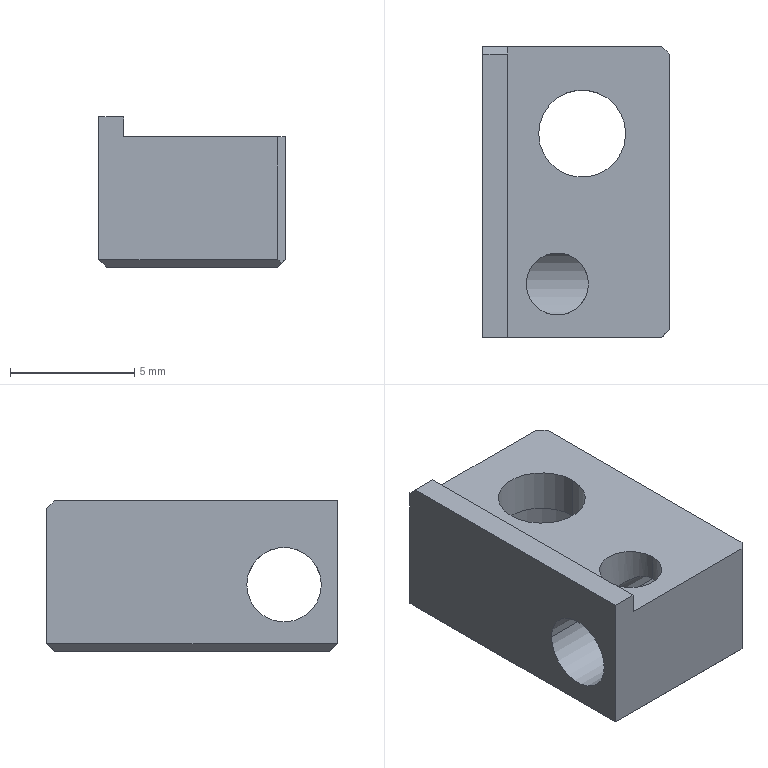Part | NX | 1 solid | 24 faces | box 7.5 x 11.687 x 6.04 mm | volume 291.783 mm3 | plane 16 | cylinder 8 | commonest cylinder face diameters 2.5 x2 3 x2 3.5 x2 6 x2
STEP:
#1=CARTESIAN_POINT('',(-53.86,-43.177,4.443));
#2=VERTEX_POINT('',#1);
#3=CARTESIAN_POINT('',(-51.36,-43.177,4.443));
#4=VERTEX_POINT('',#3);
#5=CARTESIAN_POINT('',(-52.61,-43.177,4.443));
#6=DIRECTION('',(0.,0.,1.));
#7=DIRECTION('',(1.,0.,0.));
#8=AXIS2_PLACEMENT_3D('',#5,#6,#7);
#9=CIRCLE('',#8,1.25);
#10=EDGE_CURVE('',#2,#4,#9,.T.);
#11=ORIENTED_EDGE('',*,*,#10,.T.);
#12=CARTESIAN_POINT('',(-51.36,-43.177,3.373));
#13=VERTEX_POINT('',#12);
#14=CARTESIAN_POINT('',(-51.36,-43.177,5.403));
#15=DIRECTION('',(0.,0.,1.));
#16=VECTOR('',#15,1000.);
#17=LINE('',#14,#16);
#18=EDGE_CURVE('',#13,#4,#17,.T.);
#19=ORIENTED_EDGE('',*,*,#18,.F.);
#20=CARTESIAN_POINT('',(-52.61,-44.427,2.702));
#21=VERTEX_POINT('',#20);
#22=CARTESIAN_POINT('',(-52.61,-44.427,2.702));
#23=CARTESIAN_POINT('',(-52.599,-44.427,2.702));
#24=CARTESIAN_POINT('',(-52.588,-44.426,2.702));
#25=CARTESIAN_POINT('',(-52.578,-44.426,2.703));
#26=CARTESIAN_POINT('',(-52.567,-44.426,2.703));
#27=CARTESIAN_POINT('',(-52.556,-44.425,2.704));
#28=CARTESIAN_POINT('',(-52.545,-44.425,2.705));
#29=CARTESIAN_POINT('',(-52.534,-44.424,2.706));
#30=CARTESIAN_POINT('',(-52.523,-44.424,2.707));
#31=CARTESIAN_POINT('',(-52.512,-44.423,2.708));
#32=CARTESIAN_POINT('',(-52.501,-44.422,2.709));
#33=CARTESIAN_POINT('',(-52.491,-44.421,2.711));
#34=CARTESIAN_POINT('',(-52.48,-44.42,2.712));
#35=CARTESIAN_POINT('',(-52.458,-44.418,2.716));
#36=CARTESIAN_POINT('',(-52.437,-44.415,2.72));
#37=CARTESIAN_POINT('',(-52.416,-44.411,2.725));
#38=CARTESIAN_POINT('',(-52.395,-44.408,2.73));
#39=CARTESIAN_POINT('',(-52.374,-44.404,2.735));
#40=CARTESIAN_POINT('',(-52.354,-44.4,2.741));
#41=CARTESIAN_POINT('',(-52.313,-44.391,2.753));
#42=CARTESIAN_POINT('',(-52.273,-44.381,2.768));
#43=CARTESIAN_POINT('',(-52.234,-44.369,2.784));
#44=CARTESIAN_POINT('',(-52.215,-44.363,2.792));
#45=CARTESIAN_POINT('',(-52.196,-44.356,2.8));
#46=CARTESIAN_POINT('',(-52.177,-44.349,2.809));
#47=CARTESIAN_POINT('',(-52.158,-44.342,2.817));
#48=CARTESIAN_POINT('',(-52.139,-44.335,2.826));
#49=CARTESIAN_POINT('',(-52.121,-44.327,2.836));
#50=CARTESIAN_POINT('',(-52.103,-44.319,2.845));
#51=CARTESIAN_POINT('',(-52.085,-44.311,2.854));
#52=CARTESIAN_POINT('',(-52.067,-44.303,2.864));
#53=CARTESIAN_POINT('',(-52.05,-44.294,2.874));
#54=CARTESIAN_POINT('',(-52.033,-44.285,2.884));
#55=CARTESIAN_POINT('',(-52.016,-44.276,2.893));
#56=CARTESIAN_POINT('',(-51.998,-44.267,2.903));
#57=CARTESIAN_POINT('',(-51.982,-44.257,2.913));
#58=CARTESIAN_POINT('',(-51.965,-44.247,2.924));
#59=CARTESIAN_POINT('',(-51.949,-44.237,2.934));
#60=CARTESIAN_POINT('',(-51.932,-44.227,2.944));
#61=CARTESIAN_POINT('',(-51.916,-44.216,2.954));
#62=CARTESIAN_POINT('',(-51.9,-44.205,2.965));
#63=CARTESIAN_POINT('',(-51.884,-44.194,2.975));
#64=CARTESIAN_POINT('',(-51.869,-44.183,2.985));
#65=CARTESIAN_POINT('',(-51.853,-44.171,2.996));
#66=CARTESIAN_POINT('',(-51.838,-44.16,3.006));
#67=CARTESIAN_POINT('',(-51.823,-44.147,3.017));
#68=CARTESIAN_POINT('',(-51.793,-44.123,3.037));
#69=CARTESIAN_POINT('',(-51.764,-44.097,3.058));
#70=CARTESIAN_POINT('',(-51.736,-44.07,3.078));
#71=CARTESIAN_POINT('',(-51.708,-44.043,3.098));
#72=CARTESIAN_POINT('',(-51.682,-44.014,3.118));
#73=CARTESIAN_POINT('',(-51.656,-43.985,3.137));
#74=CARTESIAN_POINT('',(-51.644,-43.97,3.146));
#75=CARTESIAN_POINT('',(-51.631,-43.954,3.156));
#76=CARTESIAN_POINT('',(-51.619,-43.939,3.165));
#77=CARTESIAN_POINT('',(-51.607,-43.923,3.174));
#78=CARTESIAN_POINT('',(-51.596,-43.907,3.183));
#79=CARTESIAN_POINT('',(-51.584,-43.891,3.192));
#80=CARTESIAN_POINT('',(-51.573,-43.874,3.201));
#81=CARTESIAN_POINT('',(-51.562,-43.857,3.21));
#82=CARTESIAN_POINT('',(-51.551,-43.84,3.218));
#83=CARTESIAN_POINT('',(-51.54,-43.823,3.227));
#84=CARTESIAN_POINT('',(-51.53,-43.806,3.235));
#85=CARTESIAN_POINT('',(-51.52,-43.788,3.243));
#86=CARTESIAN_POINT('',(-51.51,-43.77,3.251));
#87=CARTESIAN_POINT('',(-51.5,-43.752,3.259));
#88=CARTESIAN_POINT('',(-51.491,-43.733,3.266));
#89=CARTESIAN_POINT('',(-51.482,-43.715,3.273));
#90=CARTESIAN_POINT('',(-51.473,-43.696,3.28));
#91=CARTESIAN_POINT('',(-51.465,-43.677,3.287));
#92=CARTESIAN_POINT('',(-51.448,-43.639,3.301));
#93=CARTESIAN_POINT('',(-51.433,-43.6,3.313));
#94=CARTESIAN_POINT('',(-51.42,-43.56,3.323));
#95=CARTESIAN_POINT('',(-51.414,-43.539,3.329));
#96=CARTESIAN_POINT('',(-51.408,-43.519,3.334));
#97=CARTESIAN_POINT('',(-51.402,-43.498,3.338));
#98=CARTESIAN_POINT('',(-51.397,-43.478,3.343));
#99=CARTESIAN_POINT('',(-51.392,-43.457,3.347));
#100=CARTESIAN_POINT('',(-51.387,-43.436,3.351));
#101=CARTESIAN_POINT('',(-51.383,-43.414,3.354));
#102=CARTESIAN_POINT('',(-51.379,-43.393,3.358));
#103=CARTESIAN_POINT('',(-51.376,-43.372,3.36));
#104=CARTESIAN_POINT('',(-51.372,-43.35,3.363));
#105=CARTESIAN_POINT('',(-51.369,-43.329,3.366));
#106=CARTESIAN_POINT('',(-51.367,-43.307,3.367));
#107=CARTESIAN_POINT('',(-51.365,-43.285,3.369));
#108=CARTESIAN_POINT('',(-51.363,-43.264,3.371));
#109=CARTESIAN_POINT('',(-51.362,-43.242,3.372));
#110=CARTESIAN_POINT('',(-51.361,-43.22,3.373));
#111=CARTESIAN_POINT('',(-51.36,-43.198,3.373));
#112=CARTESIAN_POINT('',(-51.36,-43.177,3.373));
#113=B_SPLINE_CURVE_WITH_KNOTS('',3,(#22,#23,#24,#25,#26,#27,#28,#29,#30,#31,#32,#33,#34,#35,#36,#37,#38,#39,#40,#41,#42,#43,#44,#45,#46,#47,#48,#49,#50,#51,#52,#53,#54,#55,#56,#57,#58,#59,#60,#61,#62,#63,#64,#65,#66,#67,#68,#69,#70,#71,#72,#73,#74,#75,#76,#77,#78,#79,#80,#81,#82,#83,#84,#85,#86,#87,#88,#89,#90,#91,#92,#93,#94,#95,#96,#97,#98,#99,#100,#101,#102,#103,#104,#105,#106,#107,#108,#109,#110,#111,#112),.UNSPECIFIED.,.F.,.F.,(4,3,3,3,3,3,3,3,3,3,3,3,3,3,3,3,3,3,3,3,3,3,3,3,3,3,3,3,3,3,4),(0.,0.03265,0.06539,0.0982,0.1311,0.1968,0.2623,0.393,0.4586,0.5242,0.5897,0.655,0.7204,0.786,0.8518,0.9176,1.049,1.18,1.245,1.311,1.377,1.442,1.508,1.574,1.705,1.77,1.836,1.902,1.967,2.033,2.098),.UNSPECIFIED.);
#114=EDGE_CURVE('',#21,#13,#113,.T.);
#115=ORIENTED_EDGE('',*,*,#114,.F.);
#116=CARTESIAN_POINT('',(-53.86,-43.177,3.373));
#117=VERTEX_POINT('',#116);
#118=CARTESIAN_POINT('',(-53.86,-43.177,3.373));
#119=CARTESIAN_POINT('',(-53.86,-43.199,3.373));
#120=CARTESIAN_POINT('',(-53.86,-43.22,3.373));
#121=CARTESIAN_POINT('',(-53.859,-43.242,3.372));
#122=CARTESIAN_POINT('',(-53.857,-43.264,3.371));
#123=CARTESIAN_POINT('',(-53.856,-43.286,3.369));
#124=CARTESIAN_POINT('',(-53.853,-43.307,3.367));
#125=CARTESIAN_POINT('',(-53.851,-43.329,3.365));
#126=CARTESIAN_POINT('',(-53.848,-43.35,3.363));
#127=CARTESIAN_POINT('',(-53.845,-43.372,3.36));
#128=CARTESIAN_POINT('',(-53.842,-43.393,3.358));
#129=CARTESIAN_POINT('',(-53.838,-43.414,3.354));
#130=CARTESIAN_POINT('',(-53.833,-43.435,3.351));
#131=CARTESIAN_POINT('',(-53.829,-43.457,3.347));
#132=CARTESIAN_POINT('',(-53.824,-43.478,3.343));
#133=CARTESIAN_POINT('',(-53.818,-43.498,3.338));
#134=CARTESIAN_POINT('',(-53.813,-43.519,3.334));
#135=CARTESIAN_POINT('',(-53.807,-43.539,3.329));
#136=CARTESIAN_POINT('',(-53.8,-43.56,3.323));
#137=CARTESIAN_POINT('',(-53.794,-43.58,3.318));
#138=CARTESIAN_POINT('',(-53.787,-43.6,3.312));
#139=CARTESIAN_POINT('',(-53.779,-43.619,3.306));
#140=CARTESIAN_POINT('',(-53.772,-43.639,3.3));
#141=CARTESIAN_POINT('',(-53.764,-43.658,3.294));
#142=CARTESIAN_POINT('',(-53.756,-43.677,3.287));
#143=CARTESIAN_POINT('',(-53.747,-43.696,3.28));
#144=CARTESIAN_POINT('',(-53.739,-43.715,3.273));
#145=CARTESIAN_POINT('',(-53.73,-43.733,3.266));
#146=CARTESIAN_POINT('',(-53.72,-43.752,3.259));
#147=CARTESIAN_POINT('',(-53.711,-43.77,3.251));
#148=CARTESIAN_POINT('',(-53.701,-43.788,3.243));
#149=CARTESIAN_POINT('',(-53.691,-43.805,3.235));
#150=CARTESIAN_POINT('',(-53.68,-43.823,3.227));
#151=CARTESIAN_POINT('',(-53.67,-43.84,3.218));
#152=CARTESIAN_POINT('',(-53.659,-43.857,3.21));
#153=CARTESIAN_POINT('',(-53.648,-43.874,3.201));
#154=CARTESIAN_POINT('',(-53.636,-43.89,3.192));
#155=CARTESIAN_POINT('',(-53.625,-43.907,3.183));
#156=CARTESIAN_POINT('',(-53.613,-43.923,3.174));
#157=CARTESIAN_POINT('',(-53.601,-43.939,3.165));
#158=CARTESIAN_POINT('',(-53.589,-43.954,3.156));
#159=CARTESIAN_POINT('',(-53.577,-43.97,3.146));
#160=CARTESIAN_POINT('',(-53.564,-43.985,3.137));
#161=CARTESIAN_POINT('',(-53.539,-44.014,3.118));
#162=CARTESIAN_POINT('',(-53.512,-44.043,3.098));
#163=CARTESIAN_POINT('',(-53.485,-44.07,3.078));
#164=CARTESIAN_POINT('',(-53.457,-44.097,3.058));
#165=CARTESIAN_POINT('',(-53.428,-44.123,3.037));
#166=CARTESIAN_POINT('',(-53.398,-44.147,3.017));
#167=CARTESIAN_POINT('',(-53.383,-44.16,3.006));
#168=CARTESIAN_POINT('',(-53.367,-44.171,2.996));
#169=CARTESIAN_POINT('',(-53.352,-44.183,2.986));
#170=CARTESIAN_POINT('',(-53.336,-44.194,2.975));
#171=CARTESIAN_POINT('',(-53.32,-44.205,2.965));
#172=CARTESIAN_POINT('',(-53.304,-44.216,2.954));
#173=CARTESIAN_POINT('',(-53.288,-44.227,2.944));
#174=CARTESIAN_POINT('',(-53.272,-44.237,2.934));
#175=CARTESIAN_POINT('',(-53.255,-44.247,2.924));
#176=CARTESIAN_POINT('',(-53.239,-44.257,2.913));
#177=CARTESIAN_POINT('',(-53.222,-44.267,2.903));
#178=CARTESIAN_POINT('',(-53.205,-44.276,2.893));
#179=CARTESIAN_POINT('',(-53.188,-44.285,2.884));
#180=CARTESIAN_POINT('',(-53.171,-44.294,2.874));
#181=CARTESIAN_POINT('',(-53.153,-44.303,2.864));
#182=CARTESIAN_POINT('',(-53.135,-44.311,2.854));
#183=CARTESIAN_POINT('',(-53.117,-44.319,2.845));
#184=CARTESIAN_POINT('',(-53.099,-44.327,2.836));
#185=CARTESIAN_POINT('',(-53.081,-44.335,2.826));
#186=CARTESIAN_POINT('',(-53.063,-44.342,2.817));
#187=CARTESIAN_POINT('',(-53.044,-44.349,2.809));
#188=CARTESIAN_POINT('',(-53.025,-44.356,2.8));
#189=CARTESIAN_POINT('',(-53.006,-44.363,2.792));
#190=CARTESIAN_POINT('',(-52.986,-44.369,2.784));
#191=CARTESIAN_POINT('',(-52.948,-44.381,2.768));
#192=CARTESIAN_POINT('',(-52.908,-44.391,2.753));
#193=CARTESIAN_POINT('',(-52.867,-44.4,2.741));
#194=CARTESIAN_POINT('',(-52.846,-44.404,2.735));
#195=CARTESIAN_POINT('',(-52.826,-44.408,2.729));
#196=CARTESIAN_POINT('',(-52.804,-44.411,2.725));
#197=CARTESIAN_POINT('',(-52.783,-44.415,2.72));
#198=CARTESIAN_POINT('',(-52.762,-44.418,2.716));
#199=CARTESIAN_POINT('',(-52.74,-44.42,2.712));
#200=CARTESIAN_POINT('',(-52.73,-44.421,2.711));
#201=CARTESIAN_POINT('',(-52.719,-44.422,2.709));
#202=CARTESIAN_POINT('',(-52.708,-44.423,2.708));
#203=CARTESIAN_POINT('',(-52.697,-44.424,2.707));
#204=CARTESIAN_POINT('',(-52.686,-44.424,2.706));
#205=CARTESIAN_POINT('',(-52.675,-44.425,2.705));
#206=CARTESIAN_POINT('',(-52.665,-44.426,2.704));
#207=CARTESIAN_POINT('',(-52.654,-44.426,2.703));
#208=CARTESIAN_POINT('',(-52.643,-44.426,2.703));
#209=CARTESIAN_POINT('',(-52.632,-44.426,2.702));
#210=CARTESIAN_POINT('',(-52.621,-44.427,2.702));
#211=CARTESIAN_POINT('',(-52.61,-44.427,2.702));
#212=B_SPLINE_CURVE_WITH_KNOTS('',3,(#118,#119,#120,#121,#122,#123,#124,#125,#126,#127,#128,#129,#130,#131,#132,#133,#134,#135,#136,#137,#138,#139,#140,#141,#142,#143,#144,#145,#146,#147,#148,#149,#150,#151,#152,#153,#154,#155,#156,#157,#158,#159,#160,#161,#162,#163,#164,#165,#166,#167,#168,#169,#170,#171,#172,#173,#174,#175,#176,#177,#178,#179,#180,#181,#182,#183,#184,#185,#186,#187,#188,#189,#190,#191,#192,#193,#194,#195,#196,#197,#198,#199,#200,#201,#202,#203,#204,#205,#206,#207,#208,#209,#210,#211),.UNSPECIFIED.,.F.,.F.,(4,3,3,3,3,3,3,3,3,3,3,3,3,3,3,3,3,3,3,3,3,3,3,3,3,3,3,3,3,3,3,4),(0.,0.06564,0.131,0.1964,0.262,0.3277,0.3934,0.4588,0.5241,0.5897,0.6553,0.7211,0.7868,0.8525,0.9179,1.049,1.18,1.246,1.312,1.378,1.443,1.508,1.574,1.639,1.705,1.836,1.901,1.967,2.,2.033,2.065,2.098),.UNSPECIFIED.);
#213=EDGE_CURVE('',#117,#21,#212,.T.);
#214=ORIENTED_EDGE('',*,*,#213,.F.);
#215=CARTESIAN_POINT('',(-53.86,-43.177,5.403));
#216=DIRECTION('',(0.,0.,1.));
#217=VECTOR('',#216,1000.);
#218=LINE('',#215,#217);
#219=EDGE_CURVE('',#117,#2,#218,.T.);
#220=ORIENTED_EDGE('',*,*,#219,.T.);
#221=EDGE_LOOP('',(#11,#19,#115,#214,#220));
#222=FACE_BOUND('',#221,.T.);
#223=CARTESIAN_POINT('',(-52.61,-43.177,5.403));
#224=DIRECTION('',(0.,0.,1.));
#225=DIRECTION('',(1.,0.,0.));
#226=AXIS2_PLACEMENT_3D('',#223,#224,#225);
#227=CYLINDRICAL_SURFACE('',#226,1.25);
#228=ADVANCED_FACE('',(#222),#227,.F.);
#229=CARTESIAN_POINT('',(-55.61,-45.316,-0.4969));
#230=VERTEX_POINT('',#229);
#231=CARTESIAN_POINT('',(-55.61,-45.316,5.243));
#232=VERTEX_POINT('',#231);
#233=CARTESIAN_POINT('',(-55.61,-45.316,3.403));
#234=DIRECTION('',(0.,0.,1.));
#235=VECTOR('',#234,1000.);
#236=LINE('',#233,#235);
#237=EDGE_CURVE('',#230,#232,#236,.T.);
#238=ORIENTED_EDGE('',*,*,#237,.T.);
#239=CARTESIAN_POINT('',(-55.61,-33.929,5.243));
#240=VERTEX_POINT('',#239);
#241=CARTESIAN_POINT('',(-55.61,-36.078,5.243));
#242=DIRECTION('',(0.,1.,0.));
#243=VECTOR('',#242,1000.);
#244=LINE('',#241,#243);
#245=EDGE_CURVE('',#232,#240,#244,.T.);
#246=ORIENTED_EDGE('',*,*,#245,.T.);
#247=CARTESIAN_POINT('',(-55.61,-33.629,4.943));
#248=VERTEX_POINT('',#247);
#249=CARTESIAN_POINT('',(-55.61,-32.089,3.403));
#250=DIRECTION('',(0.,0.7071,-0.7071));
#251=VECTOR('',#250,1000.);
#252=LINE('',#249,#251);
#253=EDGE_CURVE('',#240,#248,#252,.T.);
#254=ORIENTED_EDGE('',*,*,#253,.T.);
#255=CARTESIAN_POINT('',(-55.61,-33.629,-0.4969));
#256=VERTEX_POINT('',#255);
#257=CARTESIAN_POINT('',(-55.61,-33.629,3.403));
#258=DIRECTION('',(0.,0.,1.));
#259=VECTOR('',#258,1000.);
#260=LINE('',#257,#259);
#261=EDGE_CURVE('',#256,#248,#260,.T.);
#262=ORIENTED_EDGE('',*,*,#261,.F.);
#263=CARTESIAN_POINT('',(-55.61,-39.622,-0.4969));
#264=DIRECTION('',(0.,1.,0.));
#265=VECTOR('',#264,1000.);
#266=LINE('',#263,#265);
#267=EDGE_CURVE('',#230,#256,#266,.T.);
#268=ORIENTED_EDGE('',*,*,#267,.F.);
#269=EDGE_LOOP('',(#238,#246,#254,#262,#268));
#270=FACE_BOUND('',#269,.T.);
#271=CARTESIAN_POINT('',(-55.61,-41.677,1.873));
#272=VERTEX_POINT('',#271);
#273=CARTESIAN_POINT('',(-55.61,-44.677,1.873));
#274=VERTEX_POINT('',#273);
#275=CARTESIAN_POINT('',(-55.61,-43.177,1.873));
#276=DIRECTION('',(-1.,0.,0.));
#277=DIRECTION('',(0.,-1.,0.));
#278=AXIS2_PLACEMENT_3D('',#275,#276,#277);
#279=CIRCLE('',#278,1.5);
#280=EDGE_CURVE('',#272,#274,#279,.T.);
#281=ORIENTED_EDGE('',*,*,#280,.F.);
#282=CARTESIAN_POINT('',(-55.61,-43.177,1.873));
#283=DIRECTION('',(-1.,0.,0.));
#284=DIRECTION('',(0.,-1.,0.));
#285=AXIS2_PLACEMENT_3D('',#282,#283,#284);
#286=CIRCLE('',#285,1.5);
#287=EDGE_CURVE('',#274,#272,#286,.T.);
#288=ORIENTED_EDGE('',*,*,#287,.F.);
#289=EDGE_LOOP('',(#281,#288));
#290=FACE_BOUND('',#289,.T.);
#291=CARTESIAN_POINT('',(-55.61,-32.629,3.403));
#292=DIRECTION('',(-1.,0.,0.));
#293=DIRECTION('',(0.,0.,1.));
#294=AXIS2_PLACEMENT_3D('',#291,#292,#293);
#295=PLANE('',#294);
#296=ADVANCED_FACE('',(#270,#290),#295,.T.);
#297=ORIENTED_EDGE('',*,*,#261,.T.);
#298=CARTESIAN_POINT('',(-54.61,-33.629,4.943));
#299=VERTEX_POINT('',#298);
#300=CARTESIAN_POINT('',(-55.11,-33.629,4.943));
#301=DIRECTION('',(1.,0.,0.));
#302=VECTOR('',#301,1000.);
#303=LINE('',#300,#302);
#304=EDGE_CURVE('',#248,#299,#303,.T.);
#305=ORIENTED_EDGE('',*,*,#304,.T.);
#306=CARTESIAN_POINT('',(-54.61,-33.629,4.443));
#307=VERTEX_POINT('',#306);
#308=CARTESIAN_POINT('',(-54.61,-33.629,3.403));
#309=DIRECTION('',(0.,0.,1.));
#310=VECTOR('',#309,1000.);
#311=LINE('',#308,#310);
#312=EDGE_CURVE('',#307,#299,#311,.T.);
#313=ORIENTED_EDGE('',*,*,#312,.F.);
#314=CARTESIAN_POINT('',(-48.41,-33.629,4.443));
#315=VERTEX_POINT('',#314);
#316=CARTESIAN_POINT('',(-49.386,-33.629,4.443));
#317=DIRECTION('',(-1.,0.,0.));
#318=VECTOR('',#317,1000.);
#319=LINE('',#316,#318);
#320=EDGE_CURVE('',#315,#307,#319,.T.);
#321=ORIENTED_EDGE('',*,*,#320,.F.);
#322=CARTESIAN_POINT('',(-48.41,-33.629,-0.4969));
#323=VERTEX_POINT('',#322);
#324=CARTESIAN_POINT('',(-48.41,-33.629,3.403));
#325=DIRECTION('',(0.,0.,-1.));
#326=VECTOR('',#325,1000.);
#327=LINE('',#324,#326);
#328=EDGE_CURVE('',#315,#323,#327,.T.);
#329=ORIENTED_EDGE('',*,*,#328,.T.);
#330=CARTESIAN_POINT('',(-52.01,-33.629,-0.4969));
#331=DIRECTION('',(1.,0.,0.));
#332=VECTOR('',#331,1000.);
#333=LINE('',#330,#332);
#334=EDGE_CURVE('',#256,#323,#333,.T.);
#335=ORIENTED_EDGE('',*,*,#334,.F.);
#336=EDGE_LOOP('',(#297,#305,#313,#321,#329,#335));
#337=FACE_BOUND('',#336,.T.);
#338=CARTESIAN_POINT('',(-48.11,-33.629,3.403));
#339=DIRECTION('',(0.,1.,0.));
#340=DIRECTION('',(0.,0.,-1.));
#341=AXIS2_PLACEMENT_3D('',#338,#339,#340);
#342=PLANE('',#341);
#343=ADVANCED_FACE('',(#337),#342,.T.);
#344=CARTESIAN_POINT('',(-48.11,-45.016,4.443));
#345=VERTEX_POINT('',#344);
#346=CARTESIAN_POINT('',(-48.11,-33.929,4.443));
#347=VERTEX_POINT('',#346);
#348=CARTESIAN_POINT('',(-48.11,-36.078,4.443));
#349=DIRECTION('',(0.,1.,0.));
#350=VECTOR('',#349,1000.);
#351=LINE('',#348,#350);
#352=EDGE_CURVE('',#345,#347,#351,.T.);
#353=ORIENTED_EDGE('',*,*,#352,.F.);
#354=CARTESIAN_POINT('',(-48.11,-45.016,-0.4969));
#355=VERTEX_POINT('',#354);
#356=CARTESIAN_POINT('',(-48.11,-45.016,3.403));
#357=DIRECTION('',(0.,0.,1.));
#358=VECTOR('',#357,1000.);
#359=LINE('',#356,#358);
#360=EDGE_CURVE('',#355,#345,#359,.T.);
#361=ORIENTED_EDGE('',*,*,#360,.F.);
#362=CARTESIAN_POINT('',(-48.11,-33.929,-0.4969));
#363=VERTEX_POINT('',#362);
#364=CARTESIAN_POINT('',(-48.11,-36.078,-0.4969));
#365=DIRECTION('',(0.,1.,0.));
#366=VECTOR('',#365,1000.);
#367=LINE('',#364,#366);
#368=EDGE_CURVE('',#355,#363,#367,.T.);
#369=ORIENTED_EDGE('',*,*,#368,.T.);
#370=CARTESIAN_POINT('',(-48.11,-33.929,3.403));
#371=DIRECTION('',(0.,0.,-1.));
#372=VECTOR('',#371,1000.);
#373=LINE('',#370,#372);
#374=EDGE_CURVE('',#347,#363,#373,.T.);
#375=ORIENTED_EDGE('',*,*,#374,.F.);
#376=EDGE_LOOP('',(#353,#361,#369,#375));
#377=FACE_BOUND('',#376,.T.);
#378=CARTESIAN_POINT('',(-48.11,-41.677,1.873));
#379=VERTEX_POINT('',#378);
#380=CARTESIAN_POINT('',(-48.11,-44.677,1.873));
#381=VERTEX_POINT('',#380);
#382=CARTESIAN_POINT('',(-48.11,-43.177,1.873));
#383=DIRECTION('',(-1.,0.,0.));
#384=DIRECTION('',(0.,-1.,0.));
#385=AXIS2_PLACEMENT_3D('',#382,#383,#384);
#386=CIRCLE('',#385,1.5);
#387=EDGE_CURVE('',#379,#381,#386,.T.);
#388=ORIENTED_EDGE('',*,*,#387,.T.);
#389=CARTESIAN_POINT('',(-48.11,-43.177,1.873));
#390=DIRECTION('',(-1.,0.,0.));
#391=DIRECTION('',(0.,-1.,0.));
#392=AXIS2_PLACEMENT_3D('',#389,#390,#391);
#393=CIRCLE('',#392,1.5);
#394=EDGE_CURVE('',#381,#379,#393,.T.);
#395=ORIENTED_EDGE('',*,*,#394,.T.);
#396=EDGE_LOOP('',(#388,#395));
#397=FACE_BOUND('',#396,.T.);
#398=CARTESIAN_POINT('',(-48.11,-52.629,3.403));
#399=DIRECTION('',(1.,0.,0.));
#400=DIRECTION('',(0.,0.,1.));
#401=AXIS2_PLACEMENT_3D('',#398,#399,#400);
#402=PLANE('',#401);
#403=ADVANCED_FACE('',(#377,#397),#402,.T.);
#404=ORIENTED_EDGE('',*,*,#387,.F.);
#405=CARTESIAN_POINT('',(-47.41,-41.677,1.873));
#406=DIRECTION('',(-1.,0.,0.));
#407=VECTOR('',#406,1000.);
#408=LINE('',#405,#407);
#409=EDGE_CURVE('',#272,#379,#408,.F.);
#410=ORIENTED_EDGE('',*,*,#409,.F.);
#411=ORIENTED_EDGE('',*,*,#280,.T.);
#412=CARTESIAN_POINT('',(-47.41,-44.677,1.873));
#413=DIRECTION('',(-1.,0.,0.));
#414=VECTOR('',#413,1000.);
#415=LINE('',#412,#414);
#416=EDGE_CURVE('',#274,#381,#415,.F.);
#417=ORIENTED_EDGE('',*,*,#416,.T.);
#418=EDGE_LOOP('',(#404,#410,#411,#417));
#419=FACE_BOUND('',#418,.T.);
#420=CARTESIAN_POINT('',(-47.41,-43.177,1.873));
#421=DIRECTION('',(-1.,0.,0.));
#422=DIRECTION('',(0.,-1.,0.));
#423=AXIS2_PLACEMENT_3D('',#420,#421,#422);
#424=CYLINDRICAL_SURFACE('',#423,1.5);
#425=ADVANCED_FACE('',(#419),#424,.F.);
#426=ORIENTED_EDGE('',*,*,#328,.F.);
#427=CARTESIAN_POINT('',(-49.386,-32.653,4.443));
#428=DIRECTION('',(-0.7071,0.7071,0.));
#429=VECTOR('',#428,1000.);
#430=LINE('',#427,#429);
#431=EDGE_CURVE('',#347,#315,#430,.T.);
#432=ORIENTED_EDGE('',*,*,#431,.F.);
#433=ORIENTED_EDGE('',*,*,#374,.T.);
#434=CARTESIAN_POINT('',(-48.26,-33.779,-0.6469));
#435=VERTEX_POINT('',#434);
#436=CARTESIAN_POINT('',(-49.386,-32.653,-1.773));
#437=DIRECTION('',(0.5774,-0.5774,0.5774));
#438=VECTOR('',#437,1000.);
#439=LINE('',#436,#438);
#440=EDGE_CURVE('',#435,#363,#439,.T.);
#441=ORIENTED_EDGE('',*,*,#440,.F.);
#442=CARTESIAN_POINT('',(-49.386,-32.653,0.4788));
#443=DIRECTION('',(0.5774,-0.5774,-0.5774));
#444=VECTOR('',#443,1000.);
#445=LINE('',#442,#444);
#446=EDGE_CURVE('',#323,#435,#445,.T.);
#447=ORIENTED_EDGE('',*,*,#446,.F.);
#448=EDGE_LOOP('',(#426,#432,#433,#441,#447));
#449=FACE_BOUND('',#448,.T.);
#450=CARTESIAN_POINT('',(-48.26,-33.779,1.953));
#451=DIRECTION('',(0.7071,0.7071,0.));
#452=DIRECTION('',(0.,0.,-1.));
#453=AXIS2_PLACEMENT_3D('',#450,#451,#452);
#454=PLANE('',#453);
#455=ADVANCED_FACE('',(#449),#454,.T.);
#456=CARTESIAN_POINT('',(-54.61,-33.929,5.243));
#457=VERTEX_POINT('',#456);
#458=CARTESIAN_POINT('',(-55.11,-33.929,5.243));
#459=DIRECTION('',(1.,0.,0.));
#460=VECTOR('',#459,1000.);
#461=LINE('',#458,#460);
#462=EDGE_CURVE('',#240,#457,#461,.T.);
#463=ORIENTED_EDGE('',*,*,#462,.F.);
#464=ORIENTED_EDGE('',*,*,#245,.F.);
#465=CARTESIAN_POINT('',(-54.61,-45.316,5.243));
#466=VERTEX_POINT('',#465);
#467=CARTESIAN_POINT('',(-49.386,-45.316,5.243));
#468=DIRECTION('',(-1.,0.,0.));
#469=VECTOR('',#468,1000.);
#470=LINE('',#467,#469);
#471=EDGE_CURVE('',#466,#232,#470,.T.);
#472=ORIENTED_EDGE('',*,*,#471,.F.);
#473=CARTESIAN_POINT('',(-54.61,-36.078,5.243));
#474=DIRECTION('',(0.,-1.,0.));
#475=VECTOR('',#474,1000.);
#476=LINE('',#473,#475);
#477=EDGE_CURVE('',#457,#466,#476,.T.);
#478=ORIENTED_EDGE('',*,*,#477,.F.);
#479=EDGE_LOOP('',(#463,#464,#472,#478));
#480=FACE_BOUND('',#479,.T.);
#481=CARTESIAN_POINT('',(-54.321,-38.07,5.243));
#482=DIRECTION('',(0.,0.,1.));
#483=DIRECTION('',(1.,0.,0.));
#484=AXIS2_PLACEMENT_3D('',#481,#482,#483);
#485=PLANE('',#484);
#486=ADVANCED_FACE('',(#480),#485,.T.);
#487=CARTESIAN_POINT('',(-54.61,-45.316,4.443));
#488=VERTEX_POINT('',#487);
#489=CARTESIAN_POINT('',(-54.61,-36.078,4.443));
#490=DIRECTION('',(0.,1.,0.));
#491=VECTOR('',#490,1000.);
#492=LINE('',#489,#491);
#493=EDGE_CURVE('',#488,#307,#492,.T.);
#494=ORIENTED_EDGE('',*,*,#493,.T.);
#495=ORIENTED_EDGE('',*,*,#312,.T.);
#496=CARTESIAN_POINT('',(-54.61,-32.089,3.403));
#497=DIRECTION('',(0.,-0.7071,0.7071));
#498=VECTOR('',#497,1000.);
#499=LINE('',#496,#498);
#500=EDGE_CURVE('',#299,#457,#499,.T.);
#501=ORIENTED_EDGE('',*,*,#500,.T.);
#502=ORIENTED_EDGE('',*,*,#477,.T.);
#503=CARTESIAN_POINT('',(-54.61,-45.316,3.403));
#504=DIRECTION('',(0.,0.,1.));
#505=VECTOR('',#504,1000.);
#506=LINE('',#503,#505);
#507=EDGE_CURVE('',#488,#466,#506,.T.);
#508=ORIENTED_EDGE('',*,*,#507,.F.);
#509=EDGE_LOOP('',(#494,#495,#501,#502,#508));
#510=FACE_BOUND('',#509,.T.);
#511=CARTESIAN_POINT('',(-54.61,-33.629,4.403));
#512=DIRECTION('',(1.,0.,0.));
#513=DIRECTION('',(0.,1.,0.));
#514=AXIS2_PLACEMENT_3D('',#511,#512,#513);
#515=PLANE('',#514);
#516=ADVANCED_FACE('',(#510),#515,.T.);
#517=ORIENTED_EDGE('',*,*,#462,.T.);
#518=ORIENTED_EDGE('',*,*,#500,.F.);
#519=ORIENTED_EDGE('',*,*,#304,.F.);
#520=ORIENTED_EDGE('',*,*,#253,.F.);
#521=EDGE_LOOP('',(#517,#518,#519,#520));
#522=FACE_BOUND('',#521,.T.);
#523=CARTESIAN_POINT('',(-55.11,-33.779,5.093));
#524=DIRECTION('',(0.,-0.7071,-0.7071));
#525=DIRECTION('',(0.,0.7071,-0.7071));
#526=AXIS2_PLACEMENT_3D('',#523,#524,#525);
#527=PLANE('',#526);
#528=ADVANCED_FACE('',(#522),#527,.F.);
#529=ORIENTED_EDGE('',*,*,#416,.F.);
#530=ORIENTED_EDGE('',*,*,#287,.T.);
#531=ORIENTED_EDGE('',*,*,#409,.T.);
#532=ORIENTED_EDGE('',*,*,#394,.F.);
#533=EDGE_LOOP('',(#529,#530,#531,#532));
#534=FACE_BOUND('',#533,.T.);
#535=ORIENTED_EDGE('',*,*,#213,.T.);
#536=ORIENTED_EDGE('',*,*,#114,.T.);
#537=CARTESIAN_POINT('',(-51.36,-43.177,3.373));
#538=CARTESIAN_POINT('',(-51.36,-43.148,3.373));
#539=CARTESIAN_POINT('',(-51.361,-43.12,3.372));
#540=CARTESIAN_POINT('',(-51.363,-43.092,3.371));
#541=CARTESIAN_POINT('',(-51.364,-43.077,3.37));
#542=CARTESIAN_POINT('',(-51.365,-43.062,3.369));
#543=CARTESIAN_POINT('',(-51.367,-43.047,3.367));
#544=CARTESIAN_POINT('',(-51.369,-43.032,3.366));
#545=CARTESIAN_POINT('',(-51.37,-43.017,3.365));
#546=CARTESIAN_POINT('',(-51.373,-43.002,3.363));
#547=CARTESIAN_POINT('',(-51.375,-42.987,3.361));
#548=CARTESIAN_POINT('',(-51.377,-42.972,3.359));
#549=CARTESIAN_POINT('',(-51.38,-42.957,3.357));
#550=CARTESIAN_POINT('',(-51.382,-42.942,3.355));
#551=CARTESIAN_POINT('',(-51.385,-42.928,3.352));
#552=CARTESIAN_POINT('',(-51.388,-42.913,3.35));
#553=CARTESIAN_POINT('',(-51.395,-42.884,3.345));
#554=CARTESIAN_POINT('',(-51.402,-42.855,3.339));
#555=CARTESIAN_POINT('',(-51.41,-42.827,3.332));
#556=CARTESIAN_POINT('',(-51.418,-42.798,3.325));
#557=CARTESIAN_POINT('',(-51.428,-42.771,3.317));
#558=CARTESIAN_POINT('',(-51.438,-42.743,3.309));
#559=CARTESIAN_POINT('',(-51.448,-42.716,3.301));
#560=CARTESIAN_POINT('',(-51.459,-42.689,3.292));
#561=CARTESIAN_POINT('',(-51.471,-42.662,3.282));
#562=CARTESIAN_POINT('',(-51.483,-42.636,3.273));
#563=CARTESIAN_POINT('',(-51.495,-42.611,3.262));
#564=CARTESIAN_POINT('',(-51.509,-42.586,3.252));
#565=CARTESIAN_POINT('',(-51.516,-42.573,3.246));
#566=CARTESIAN_POINT('',(-51.522,-42.561,3.241));
#567=CARTESIAN_POINT('',(-51.529,-42.549,3.235));
#568=CARTESIAN_POINT('',(-51.536,-42.537,3.23));
#569=CARTESIAN_POINT('',(-51.544,-42.525,3.224));
#570=CARTESIAN_POINT('',(-51.551,-42.513,3.218));
#571=CARTESIAN_POINT('',(-51.566,-42.489,3.206));
#572=CARTESIAN_POINT('',(-51.582,-42.466,3.194));
#573=CARTESIAN_POINT('',(-51.598,-42.444,3.182));
#574=CARTESIAN_POINT('',(-51.616,-42.419,3.168));
#575=CARTESIAN_POINT('',(-51.635,-42.394,3.153));
#576=CARTESIAN_POINT('',(-51.654,-42.371,3.138));
#577=CARTESIAN_POINT('',(-51.674,-42.348,3.124));
#578=CARTESIAN_POINT('',(-51.695,-42.325,3.108));
#579=CARTESIAN_POINT('',(-51.716,-42.304,3.093));
#580=CARTESIAN_POINT('',(-51.737,-42.282,3.077));
#581=CARTESIAN_POINT('',(-51.758,-42.261,3.062));
#582=CARTESIAN_POINT('',(-51.781,-42.241,3.046));
#583=CARTESIAN_POINT('',(-51.792,-42.232,3.038));
#584=CARTESIAN_POINT('',(-51.803,-42.222,3.03));
#585=CARTESIAN_POINT('',(-51.815,-42.212,3.022));
#586=CARTESIAN_POINT('',(-51.826,-42.203,3.014));
#587=CARTESIAN_POINT('',(-51.838,-42.194,3.006));
#588=CARTESIAN_POINT('',(-51.85,-42.185,2.998));
#589=CARTESIAN_POINT('',(-51.873,-42.166,2.982));
#590=CARTESIAN_POINT('',(-51.898,-42.149,2.966));
#591=CARTESIAN_POINT('',(-51.923,-42.133,2.95));
#592=CARTESIAN_POINT('',(-51.948,-42.116,2.934));
#593=CARTESIAN_POINT('',(-51.973,-42.101,2.918));
#594=CARTESIAN_POINT('',(-52.,-42.086,2.903));
#595=CARTESIAN_POINT('',(-52.026,-42.071,2.887));
#596=CARTESIAN_POINT('',(-52.053,-42.057,2.872));
#597=CARTESIAN_POINT('',(-52.081,-42.044,2.857));
#598=CARTESIAN_POINT('',(-52.108,-42.032,2.842));
#599=CARTESIAN_POINT('',(-52.136,-42.02,2.828));
#600=CARTESIAN_POINT('',(-52.165,-42.009,2.814));
#601=CARTESIAN_POINT('',(-52.182,-42.002,2.806));
#602=CARTESIAN_POINT('',(-52.199,-41.996,2.799));
#603=CARTESIAN_POINT('',(-52.216,-41.99,2.791));
#604=CARTESIAN_POINT('',(-52.233,-41.985,2.784));
#605=CARTESIAN_POINT('',(-52.251,-41.979,2.777));
#606=CARTESIAN_POINT('',(-52.269,-41.974,2.77));
#607=CARTESIAN_POINT('',(-52.286,-41.969,2.763));
#608=CARTESIAN_POINT('',(-52.304,-41.964,2.757));
#609=CARTESIAN_POINT('',(-52.323,-41.96,2.751));
#610=CARTESIAN_POINT('',(-52.341,-41.956,2.745));
#611=CARTESIAN_POINT('',(-52.36,-41.952,2.739));
#612=CARTESIAN_POINT('',(-52.378,-41.948,2.734));
#613=CARTESIAN_POINT('',(-52.397,-41.945,2.729));
#614=CARTESIAN_POINT('',(-52.416,-41.942,2.725));
#615=CARTESIAN_POINT('',(-52.435,-41.939,2.721));
#616=CARTESIAN_POINT('',(-52.454,-41.936,2.717));
#617=CARTESIAN_POINT('',(-52.473,-41.934,2.713));
#618=CARTESIAN_POINT('',(-52.492,-41.932,2.711));
#619=CARTESIAN_POINT('',(-52.512,-41.93,2.708));
#620=CARTESIAN_POINT('',(-52.531,-41.929,2.706));
#621=CARTESIAN_POINT('',(-52.551,-41.928,2.704));
#622=CARTESIAN_POINT('',(-52.57,-41.927,2.703));
#623=CARTESIAN_POINT('',(-52.59,-41.927,2.702));
#624=CARTESIAN_POINT('',(-52.61,-41.927,2.702));
#625=CARTESIAN_POINT('',(-52.63,-41.927,2.702));
#626=CARTESIAN_POINT('',(-52.649,-41.927,2.703));
#627=CARTESIAN_POINT('',(-52.669,-41.928,2.704));
#628=CARTESIAN_POINT('',(-52.689,-41.929,2.706));
#629=CARTESIAN_POINT('',(-52.708,-41.93,2.708));
#630=CARTESIAN_POINT('',(-52.728,-41.932,2.711));
#631=CARTESIAN_POINT('',(-52.747,-41.934,2.713));
#632=CARTESIAN_POINT('',(-52.766,-41.936,2.717));
#633=CARTESIAN_POINT('',(-52.785,-41.939,2.72));
#634=CARTESIAN_POINT('',(-52.804,-41.942,2.724));
#635=CARTESIAN_POINT('',(-52.823,-41.945,2.729));
#636=CARTESIAN_POINT('',(-52.842,-41.948,2.734));
#637=CARTESIAN_POINT('',(-52.86,-41.952,2.739));
#638=CARTESIAN_POINT('',(-52.879,-41.956,2.744));
#639=CARTESIAN_POINT('',(-52.897,-41.96,2.75));
#640=CARTESIAN_POINT('',(-52.915,-41.964,2.756));
#641=CARTESIAN_POINT('',(-52.933,-41.969,2.763));
#642=CARTESIAN_POINT('',(-52.951,-41.974,2.77));
#643=CARTESIAN_POINT('',(-52.969,-41.979,2.776));
#644=CARTESIAN_POINT('',(-52.987,-41.984,2.783));
#645=CARTESIAN_POINT('',(-53.004,-41.99,2.791));
#646=CARTESIAN_POINT('',(-53.021,-41.996,2.798));
#647=CARTESIAN_POINT('',(-53.038,-42.002,2.806));
#648=CARTESIAN_POINT('',(-53.055,-42.008,2.814));
#649=CARTESIAN_POINT('',(-53.084,-42.019,2.827));
#650=CARTESIAN_POINT('',(-53.112,-42.031,2.842));
#651=CARTESIAN_POINT('',(-53.139,-42.044,2.857));
#652=CARTESIAN_POINT('',(-53.167,-42.057,2.871));
#653=CARTESIAN_POINT('',(-53.194,-42.071,2.887));
#654=CARTESIAN_POINT('',(-53.22,-42.086,2.902));
#655=CARTESIAN_POINT('',(-53.246,-42.1,2.918));
#656=CARTESIAN_POINT('',(-53.272,-42.116,2.934));
#657=CARTESIAN_POINT('',(-53.297,-42.132,2.95));
#658=CARTESIAN_POINT('',(-53.322,-42.149,2.966));
#659=CARTESIAN_POINT('',(-53.346,-42.166,2.982));
#660=CARTESIAN_POINT('',(-53.37,-42.184,2.998));
#661=CARTESIAN_POINT('',(-53.382,-42.193,3.006));
#662=CARTESIAN_POINT('',(-53.394,-42.202,3.014));
#663=CARTESIAN_POINT('',(-53.405,-42.212,3.022));
#664=CARTESIAN_POINT('',(-53.417,-42.221,3.03));
#665=CARTESIAN_POINT('',(-53.428,-42.231,3.038));
#666=CARTESIAN_POINT('',(-53.439,-42.241,3.045));
#667=CARTESIAN_POINT('',(-53.461,-42.261,3.061));
#668=CARTESIAN_POINT('',(-53.483,-42.281,3.077));
#669=CARTESIAN_POINT('',(-53.504,-42.303,3.092));
#670=CARTESIAN_POINT('',(-53.525,-42.325,3.108));
#671=CARTESIAN_POINT('',(-53.546,-42.347,3.123));
#672=CARTESIAN_POINT('',(-53.566,-42.371,3.138));
#673=CARTESIAN_POINT('',(-53.585,-42.394,3.153));
#674=CARTESIAN_POINT('',(-53.604,-42.418,3.167));
#675=CARTESIAN_POINT('',(-53.622,-42.443,3.182));
#676=CARTESIAN_POINT('',(-53.639,-42.466,3.194));
#677=CARTESIAN_POINT('',(-53.654,-42.489,3.206));
#678=CARTESIAN_POINT('',(-53.669,-42.512,3.218));
#679=CARTESIAN_POINT('',(-53.684,-42.536,3.23));
#680=CARTESIAN_POINT('',(-53.698,-42.56,3.241));
#681=CARTESIAN_POINT('',(-53.711,-42.585,3.252));
#682=CARTESIAN_POINT('',(-53.725,-42.61,3.262));
#683=CARTESIAN_POINT('',(-53.737,-42.636,3.272));
#684=CARTESIAN_POINT('',(-53.749,-42.662,3.282));
#685=CARTESIAN_POINT('',(-53.761,-42.688,3.292));
#686=CARTESIAN_POINT('',(-53.772,-42.715,3.301));
#687=CARTESIAN_POINT('',(-53.782,-42.743,3.309));
#688=CARTESIAN_POINT('',(-53.793,-42.77,3.317));
#689=CARTESIAN_POINT('',(-53.802,-42.798,3.325));
#690=CARTESIAN_POINT('',(-53.81,-42.826,3.332));
#691=CARTESIAN_POINT('',(-53.819,-42.855,3.338));
#692=CARTESIAN_POINT('',(-53.826,-42.884,3.345));
#693=CARTESIAN_POINT('',(-53.832,-42.913,3.35));
#694=CARTESIAN_POINT('',(-53.835,-42.928,3.352));
#695=CARTESIAN_POINT('',(-53.838,-42.942,3.355));
#696=CARTESIAN_POINT('',(-53.841,-42.957,3.357));
#697=CARTESIAN_POINT('',(-53.843,-42.972,3.359));
#698=CARTESIAN_POINT('',(-53.846,-42.986,3.361));
#699=CARTESIAN_POINT('',(-53.848,-43.001,3.363));
#700=CARTESIAN_POINT('',(-53.85,-43.016,3.365));
#701=CARTESIAN_POINT('',(-53.852,-43.031,3.366));
#702=CARTESIAN_POINT('',(-53.853,-43.046,3.367));
#703=CARTESIAN_POINT('',(-53.855,-43.061,3.369));
#704=CARTESIAN_POINT('',(-53.856,-43.076,3.37));
#705=CARTESIAN_POINT('',(-53.857,-43.091,3.371));
#706=CARTESIAN_POINT('',(-53.859,-43.12,3.372));
#707=CARTESIAN_POINT('',(-53.86,-43.148,3.373));
#708=CARTESIAN_POINT('',(-53.86,-43.177,3.373));
#709=B_SPLINE_CURVE_WITH_KNOTS('',3,(#537,#538,#539,#540,#541,#542,#543,#544,#545,#546,#547,#548,#549,#550,#551,#552,#553,#554,#555,#556,#557,#558,#559,#560,#561,#562,#563,#564,#565,#566,#567,#568,#569,#570,#571,#572,#573,#574,#575,#576,#577,#578,#579,#580,#581,#582,#583,#584,#585,#586,#587,#588,#589,#590,#591,#592,#593,#594,#595,#596,#597,#598,#599,#600,#601,#602,#603,#604,#605,#606,#607,#608,#609,#610,#611,#612,#613,#614,#615,#616,#617,#618,#619,#620,#621,#622,#623,#624,#625,#626,#627,#628,#629,#630,#631,#632,#633,#634,#635,#636,#637,#638,#639,#640,#641,#642,#643,#644,#645,#646,#647,#648,#649,#650,#651,#652,#653,#654,#655,#656,#657,#658,#659,#660,#661,#662,#663,#664,#665,#666,#667,#668,#669,#670,#671,#672,#673,#674,#675,#676,#677,#678,#679,#680,#681,#682,#683,#684,#685,#686,#687,#688,#689,#690,#691,#692,#693,#694,#695,#696,#697,#698,#699,#700,#701,#702,#703,#704,#705,#706,#707,#708),.UNSPECIFIED.,.F.,.F.,(4,3,3,3,3,3,3,3,3,3,3,3,3,3,3,3,3,3,3,3,3,3,3,3,3,3,3,3,3,3,3,3,3,3,3,3,3,3,3,3,3,3,3,3,3,3,3,3,3,3,3,3,3,3,3,3,3,4),(0.,0.08477,0.1304,0.176,0.2215,0.2669,0.3577,0.4488,0.54,0.631,0.6763,0.7217,0.8127,0.9145,1.016,1.118,1.169,1.219,1.321,1.423,1.524,1.626,1.685,1.744,1.803,1.862,1.921,1.98,2.038,2.098,2.157,2.216,2.275,2.334,2.393,2.452,2.511,2.57,2.671,2.772,2.874,2.976,3.027,3.077,3.179,3.281,3.383,3.474,3.565,3.655,3.747,3.838,3.929,3.974,4.02,4.065,4.111,4.196),.UNSPECIFIED.);
#710=EDGE_CURVE('',#13,#117,#709,.T.);
#711=ORIENTED_EDGE('',*,*,#710,.T.);
#712=EDGE_LOOP('',(#535,#536,#711));
#713=FACE_BOUND('',#712,.T.);
#714=CARTESIAN_POINT('',(-47.41,-43.177,1.873));
#715=DIRECTION('',(-1.,0.,0.));
#716=DIRECTION('',(0.,-1.,0.));
#717=AXIS2_PLACEMENT_3D('',#714,#715,#716);
#718=CYLINDRICAL_SURFACE('',#717,1.5);
#719=ADVANCED_FACE('',(#534,#713),#718,.F.);
#720=ORIENTED_EDGE('',*,*,#18,.T.);
#721=CARTESIAN_POINT('',(-52.61,-43.177,4.443));
#722=DIRECTION('',(0.,0.,1.));
#723=DIRECTION('',(1.,0.,0.));
#724=AXIS2_PLACEMENT_3D('',#721,#722,#723);
#725=CIRCLE('',#724,1.25);
#726=EDGE_CURVE('',#4,#2,#725,.T.);
#727=ORIENTED_EDGE('',*,*,#726,.T.);
#728=ORIENTED_EDGE('',*,*,#219,.F.);
#729=ORIENTED_EDGE('',*,*,#710,.F.);
#730=EDGE_LOOP('',(#720,#727,#728,#729));
#731=FACE_BOUND('',#730,.T.);
#732=CARTESIAN_POINT('',(-52.61,-43.177,5.403));
#733=DIRECTION('',(0.,0.,1.));
#734=DIRECTION('',(1.,0.,0.));
#735=AXIS2_PLACEMENT_3D('',#732,#733,#734);
#736=CYLINDRICAL_SURFACE('',#735,1.25);
#737=ADVANCED_FACE('',(#731),#736,.F.);
#738=CARTESIAN_POINT('',(-55.31,-45.016,-0.7969));
#739=VERTEX_POINT('',#738);
#740=CARTESIAN_POINT('',(-55.31,-33.929,-0.7969));
#741=VERTEX_POINT('',#740);
#742=CARTESIAN_POINT('',(-55.31,-39.622,-0.7969));
#743=DIRECTION('',(0.,1.,0.));
#744=VECTOR('',#743,1000.);
#745=LINE('',#742,#744);
#746=EDGE_CURVE('',#739,#741,#745,.T.);
#747=ORIENTED_EDGE('',*,*,#746,.T.);
#748=CARTESIAN_POINT('',(-48.41,-33.929,-0.7969));
#749=VERTEX_POINT('',#748);
#750=CARTESIAN_POINT('',(-49.386,-33.929,-0.7969));
#751=DIRECTION('',(1.,0.,0.));
#752=VECTOR('',#751,1000.);
#753=LINE('',#750,#752);
#754=EDGE_CURVE('',#741,#749,#753,.T.);
#755=ORIENTED_EDGE('',*,*,#754,.T.);
#756=CARTESIAN_POINT('',(-48.41,-45.016,-0.7969));
#757=VERTEX_POINT('',#756);
#758=CARTESIAN_POINT('',(-48.41,-36.078,-0.7969));
#759=DIRECTION('',(0.,1.,0.));
#760=VECTOR('',#759,1000.);
#761=LINE('',#758,#760);
#762=EDGE_CURVE('',#757,#749,#761,.T.);
#763=ORIENTED_EDGE('',*,*,#762,.F.);
#764=CARTESIAN_POINT('',(-52.01,-45.016,-0.7969));
#765=DIRECTION('',(-1.,0.,0.));
#766=VECTOR('',#765,1000.);
#767=LINE('',#764,#766);
#768=EDGE_CURVE('',#757,#739,#767,.T.);
#769=ORIENTED_EDGE('',*,*,#768,.T.);
#770=EDGE_LOOP('',(#747,#755,#763,#769));
#771=FACE_BOUND('',#770,.T.);
#772=CARTESIAN_POINT('',(-48.61,-37.129,-0.7969));
#773=VERTEX_POINT('',#772);
#774=CARTESIAN_POINT('',(-54.61,-37.129,-0.7969));
#775=VERTEX_POINT('',#774);
#776=CARTESIAN_POINT('',(-51.61,-37.129,-0.7969));
#777=DIRECTION('',(0.,0.,-1.));
#778=DIRECTION('',(-1.,0.,0.));
#779=AXIS2_PLACEMENT_3D('',#776,#777,#778);
#780=CIRCLE('',#779,3.);
#781=EDGE_CURVE('',#773,#775,#780,.T.);
#782=ORIENTED_EDGE('',*,*,#781,.F.);
#783=CARTESIAN_POINT('',(-51.61,-37.129,-0.7969));
#784=DIRECTION('',(0.,0.,-1.));
#785=DIRECTION('',(-1.,0.,0.));
#786=AXIS2_PLACEMENT_3D('',#783,#784,#785);
#787=CIRCLE('',#786,3.);
#788=EDGE_CURVE('',#775,#773,#787,.T.);
#789=ORIENTED_EDGE('',*,*,#788,.F.);
#790=EDGE_LOOP('',(#782,#789));
#791=FACE_BOUND('',#790,.T.);
#792=CARTESIAN_POINT('',(-49.386,-36.078,-0.7969));
#793=DIRECTION('',(0.,0.,-1.));
#794=DIRECTION('',(0.,-1.,0.));
#795=AXIS2_PLACEMENT_3D('',#792,#793,#794);
#796=PLANE('',#795);
#797=ADVANCED_FACE('',(#771,#791),#796,.T.);
#798=CARTESIAN_POINT('',(-48.41,-45.316,-0.4969));
#799=VERTEX_POINT('',#798);
#800=CARTESIAN_POINT('',(-52.01,-45.316,-0.4969));
#801=DIRECTION('',(-1.,0.,0.));
#802=VECTOR('',#801,1000.);
#803=LINE('',#800,#802);
#804=EDGE_CURVE('',#799,#230,#803,.T.);
#805=ORIENTED_EDGE('',*,*,#804,.F.);
#806=CARTESIAN_POINT('',(-48.41,-45.316,4.443));
#807=VERTEX_POINT('',#806);
#808=CARTESIAN_POINT('',(-48.41,-45.316,3.403));
#809=DIRECTION('',(0.,0.,1.));
#810=VECTOR('',#809,1000.);
#811=LINE('',#808,#810);
#812=EDGE_CURVE('',#799,#807,#811,.T.);
#813=ORIENTED_EDGE('',*,*,#812,.T.);
#814=CARTESIAN_POINT('',(-49.386,-45.316,4.443));
#815=DIRECTION('',(1.,0.,0.));
#816=VECTOR('',#815,1000.);
#817=LINE('',#814,#816);
#818=EDGE_CURVE('',#488,#807,#817,.T.);
#819=ORIENTED_EDGE('',*,*,#818,.F.);
#820=ORIENTED_EDGE('',*,*,#507,.T.);
#821=ORIENTED_EDGE('',*,*,#471,.T.);
#822=ORIENTED_EDGE('',*,*,#237,.F.);
#823=EDGE_LOOP('',(#805,#813,#819,#820,#821,#822));
#824=FACE_BOUND('',#823,.T.);
#825=CARTESIAN_POINT('',(-33.55,-45.316,3.403));
#826=DIRECTION('',(0.,-1.,0.));
#827=DIRECTION('',(-1.,0.,0.));
#828=AXIS2_PLACEMENT_3D('',#825,#826,#827);
#829=PLANE('',#828);
#830=ADVANCED_FACE('',(#824),#829,.T.);
#831=ORIENTED_EDGE('',*,*,#493,.F.);
#832=ORIENTED_EDGE('',*,*,#818,.T.);
#833=CARTESIAN_POINT('',(-49.386,-46.292,4.443));
#834=DIRECTION('',(0.7071,0.7071,0.));
#835=VECTOR('',#834,1000.);
#836=LINE('',#833,#835);
#837=EDGE_CURVE('',#807,#345,#836,.T.);
#838=ORIENTED_EDGE('',*,*,#837,.T.);
#839=ORIENTED_EDGE('',*,*,#352,.T.);
#840=ORIENTED_EDGE('',*,*,#431,.T.);
#841=ORIENTED_EDGE('',*,*,#320,.T.);
#842=EDGE_LOOP('',(#831,#832,#838,#839,#840,#841));
#843=FACE_BOUND('',#842,.T.);
#844=CARTESIAN_POINT('',(-49.86,-37.129,4.443));
#845=VERTEX_POINT('',#844);
#846=CARTESIAN_POINT('',(-53.36,-37.129,4.443));
#847=VERTEX_POINT('',#846);
#848=CARTESIAN_POINT('',(-51.61,-37.129,4.443));
#849=DIRECTION('',(0.,0.,-1.));
#850=DIRECTION('',(-1.,0.,0.));
#851=AXIS2_PLACEMENT_3D('',#848,#849,#850);
#852=CIRCLE('',#851,1.75);
#853=EDGE_CURVE('',#845,#847,#852,.T.);
#854=ORIENTED_EDGE('',*,*,#853,.T.);
#855=CARTESIAN_POINT('',(-51.61,-37.129,4.443));
#856=DIRECTION('',(0.,0.,-1.));
#857=DIRECTION('',(-1.,0.,0.));
#858=AXIS2_PLACEMENT_3D('',#855,#856,#857);
#859=CIRCLE('',#858,1.75);
#860=EDGE_CURVE('',#847,#845,#859,.T.);
#861=ORIENTED_EDGE('',*,*,#860,.T.);
#862=EDGE_LOOP('',(#854,#861));
#863=FACE_BOUND('',#862,.T.);
#864=ORIENTED_EDGE('',*,*,#10,.F.);
#865=ORIENTED_EDGE('',*,*,#726,.F.);
#866=EDGE_LOOP('',(#864,#865));
#867=FACE_BOUND('',#866,.T.);
#868=CARTESIAN_POINT('',(-49.386,-36.078,4.443));
#869=DIRECTION('',(0.,0.,-1.));
#870=DIRECTION('',(0.,-1.,0.));
#871=AXIS2_PLACEMENT_3D('',#868,#869,#870);
#872=PLANE('',#871);
#873=ADVANCED_FACE('',(#843,#863,#867),#872,.F.);
#874=CARTESIAN_POINT('',(-53.161,-36.078,-2.946));
#875=DIRECTION('',(0.5774,-0.5774,-0.5774));
#876=VECTOR('',#875,1000.);
#877=LINE('',#874,#876);
#878=EDGE_CURVE('',#256,#741,#877,.T.);
#879=ORIENTED_EDGE('',*,*,#878,.F.);
#880=ORIENTED_EDGE('',*,*,#334,.T.);
#881=ORIENTED_EDGE('',*,*,#446,.T.);
#882=CARTESIAN_POINT('',(-49.386,-34.905,-1.773));
#883=DIRECTION('',(0.5774,0.5774,0.5774));
#884=VECTOR('',#883,1000.);
#885=LINE('',#882,#884);
#886=EDGE_CURVE('',#749,#435,#885,.T.);
#887=ORIENTED_EDGE('',*,*,#886,.F.);
#888=ORIENTED_EDGE('',*,*,#754,.F.);
#889=EDGE_LOOP('',(#879,#880,#881,#887,#888));
#890=FACE_BOUND('',#889,.T.);
#891=CARTESIAN_POINT('',(-52.01,-33.779,-0.6469));
#892=DIRECTION('',(0.,0.7071,-0.7071));
#893=DIRECTION('',(-1.,0.,0.));
#894=AXIS2_PLACEMENT_3D('',#891,#892,#893);
#895=PLANE('',#894);
#896=ADVANCED_FACE('',(#890),#895,.T.);
#897=ORIENTED_EDGE('',*,*,#812,.F.);
#898=CARTESIAN_POINT('',(-48.26,-45.166,-0.6469));
#899=VERTEX_POINT('',#898);
#900=CARTESIAN_POINT('',(-49.386,-46.292,0.4788));
#901=DIRECTION('',(-0.5774,-0.5774,0.5774));
#902=VECTOR('',#901,1000.);
#903=LINE('',#900,#902);
#904=EDGE_CURVE('',#899,#799,#903,.T.);
#905=ORIENTED_EDGE('',*,*,#904,.F.);
#906=CARTESIAN_POINT('',(-49.386,-46.292,-1.773));
#907=DIRECTION('',(-0.5774,-0.5774,-0.5774));
#908=VECTOR('',#907,1000.);
#909=LINE('',#906,#908);
#910=EDGE_CURVE('',#355,#899,#909,.T.);
#911=ORIENTED_EDGE('',*,*,#910,.F.);
#912=ORIENTED_EDGE('',*,*,#360,.T.);
#913=ORIENTED_EDGE('',*,*,#837,.F.);
#914=EDGE_LOOP('',(#897,#905,#911,#912,#913));
#915=FACE_BOUND('',#914,.T.);
#916=CARTESIAN_POINT('',(-48.26,-45.166,1.953));
#917=DIRECTION('',(0.7071,-0.7071,0.));
#918=DIRECTION('',(0.,0.,-1.));
#919=AXIS2_PLACEMENT_3D('',#916,#917,#918);
#920=PLANE('',#919);
#921=ADVANCED_FACE('',(#915),#920,.T.);
#922=ORIENTED_EDGE('',*,*,#762,.T.);
#923=ORIENTED_EDGE('',*,*,#886,.T.);
#924=ORIENTED_EDGE('',*,*,#440,.T.);
#925=ORIENTED_EDGE('',*,*,#368,.F.);
#926=ORIENTED_EDGE('',*,*,#910,.T.);
#927=CARTESIAN_POINT('',(-57.348,-36.078,-9.735));
#928=DIRECTION('',(-0.5774,0.5774,-0.5774));
#929=VECTOR('',#928,1000.);
#930=LINE('',#927,#929);
#931=EDGE_CURVE('',#899,#757,#930,.T.);
#932=ORIENTED_EDGE('',*,*,#931,.T.);
#933=EDGE_LOOP('',(#922,#923,#924,#925,#926,#932));
#934=FACE_BOUND('',#933,.T.);
#935=CARTESIAN_POINT('',(-48.26,-38.972,-0.6469));
#936=DIRECTION('',(-0.7071,0.,0.7071));
#937=DIRECTION('',(0.,1.,0.));
#938=AXIS2_PLACEMENT_3D('',#935,#936,#937);
#939=PLANE('',#938);
#940=ADVANCED_FACE('',(#934),#939,.F.);
#941=ORIENTED_EDGE('',*,*,#768,.F.);
#942=ORIENTED_EDGE('',*,*,#931,.F.);
#943=ORIENTED_EDGE('',*,*,#904,.T.);
#944=ORIENTED_EDGE('',*,*,#804,.T.);
#945=CARTESIAN_POINT('',(-49.386,-39.092,-6.721));
#946=DIRECTION('',(0.5774,0.5774,-0.5774));
#947=VECTOR('',#946,1000.);
#948=LINE('',#945,#947);
#949=EDGE_CURVE('',#230,#739,#948,.T.);
#950=ORIENTED_EDGE('',*,*,#949,.T.);
#951=EDGE_LOOP('',(#941,#942,#943,#944,#950));
#952=FACE_BOUND('',#951,.T.);
#953=CARTESIAN_POINT('',(-52.01,-45.166,-0.6469));
#954=DIRECTION('',(0.,-0.7071,-0.7071));
#955=DIRECTION('',(0.,-0.7071,0.7071));
#956=AXIS2_PLACEMENT_3D('',#953,#954,#955);
#957=PLANE('',#956);
#958=ADVANCED_FACE('',(#952),#957,.T.);
#959=ORIENTED_EDGE('',*,*,#746,.F.);
#960=ORIENTED_EDGE('',*,*,#949,.F.);
#961=ORIENTED_EDGE('',*,*,#267,.T.);
#962=ORIENTED_EDGE('',*,*,#878,.T.);
#963=EDGE_LOOP('',(#959,#960,#961,#962));
#964=FACE_BOUND('',#963,.T.);
#965=CARTESIAN_POINT('',(-55.46,-39.622,-0.6469));
#966=DIRECTION('',(-0.7071,0.,-0.7071));
#967=DIRECTION('',(-0.7071,0.,0.7071));
#968=AXIS2_PLACEMENT_3D('',#965,#966,#967);
#969=PLANE('',#968);
#970=ADVANCED_FACE('',(#964),#969,.T.);
#971=ORIENTED_EDGE('',*,*,#781,.T.);
#972=CARTESIAN_POINT('',(-54.61,-37.129,2.703));
#973=VERTEX_POINT('',#972);
#974=CARTESIAN_POINT('',(-54.61,-37.129,-1.597));
#975=DIRECTION('',(0.,0.,-1.));
#976=VECTOR('',#975,1000.);
#977=LINE('',#974,#976);
#978=EDGE_CURVE('',#775,#973,#977,.F.);
#979=ORIENTED_EDGE('',*,*,#978,.T.);
#980=CARTESIAN_POINT('',(-48.61,-37.129,2.703));
#981=VERTEX_POINT('',#980);
#982=CARTESIAN_POINT('',(-51.61,-37.129,2.703));
#983=DIRECTION('',(0.,0.,-1.));
#984=DIRECTION('',(-1.,0.,0.));
#985=AXIS2_PLACEMENT_3D('',#982,#983,#984);
#986=CIRCLE('',#985,3.);
#987=EDGE_CURVE('',#981,#973,#986,.T.);
#988=ORIENTED_EDGE('',*,*,#987,.F.);
#989=CARTESIAN_POINT('',(-48.61,-37.129,-1.597));
#990=DIRECTION('',(0.,0.,-1.));
#991=VECTOR('',#990,1000.);
#992=LINE('',#989,#991);
#993=EDGE_CURVE('',#773,#981,#992,.F.);
#994=ORIENTED_EDGE('',*,*,#993,.F.);
#995=EDGE_LOOP('',(#971,#979,#988,#994));
#996=FACE_BOUND('',#995,.T.);
#997=CARTESIAN_POINT('',(-51.61,-37.129,-1.597));
#998=DIRECTION('',(0.,0.,-1.));
#999=DIRECTION('',(-1.,0.,0.));
#1000=AXIS2_PLACEMENT_3D('',#997,#998,#999);
#1001=CYLINDRICAL_SURFACE('',#1000,3.);
#1002=ADVANCED_FACE('',(#996),#1001,.F.);
#1003=ORIENTED_EDGE('',*,*,#987,.T.);
#1004=CARTESIAN_POINT('',(-51.61,-37.129,2.703));
#1005=DIRECTION('',(0.,0.,-1.));
#1006=DIRECTION('',(-1.,0.,0.));
#1007=AXIS2_PLACEMENT_3D('',#1004,#1005,#1006);
#1008=CIRCLE('',#1007,3.);
#1009=EDGE_CURVE('',#973,#981,#1008,.T.);
#1010=ORIENTED_EDGE('',*,*,#1009,.T.);
#1011=EDGE_LOOP('',(#1003,#1010));
#1012=FACE_BOUND('',#1011,.T.);
#1013=CARTESIAN_POINT('',(-49.86,-37.129,2.703));
#1014=VERTEX_POINT('',#1013);
#1015=CARTESIAN_POINT('',(-53.36,-37.129,2.703));
#1016=VERTEX_POINT('',#1015);
#1017=CARTESIAN_POINT('',(-51.61,-37.129,2.703));
#1018=DIRECTION('',(0.,0.,-1.));
#1019=DIRECTION('',(-1.,0.,0.));
#1020=AXIS2_PLACEMENT_3D('',#1017,#1018,#1019);
#1021=CIRCLE('',#1020,1.75);
#1022=EDGE_CURVE('',#1014,#1016,#1021,.T.);
#1023=ORIENTED_EDGE('',*,*,#1022,.F.);
#1024=CARTESIAN_POINT('',(-51.61,-37.129,2.703));
#1025=DIRECTION('',(0.,0.,-1.));
#1026=DIRECTION('',(-1.,0.,0.));
#1027=AXIS2_PLACEMENT_3D('',#1024,#1025,#1026);
#1028=CIRCLE('',#1027,1.75);
#1029=EDGE_CURVE('',#1016,#1014,#1028,.T.);
#1030=ORIENTED_EDGE('',*,*,#1029,.F.);
#1031=EDGE_LOOP('',(#1023,#1030));
#1032=FACE_BOUND('',#1031,.T.);
#1033=CARTESIAN_POINT('',(-51.61,-37.129,2.703));
#1034=DIRECTION('',(0.,0.,-1.));
#1035=DIRECTION('',(0.,-1.,0.));
#1036=AXIS2_PLACEMENT_3D('',#1033,#1034,#1035);
#1037=PLANE('',#1036);
#1038=ADVANCED_FACE('',(#1012,#1032),#1037,.T.);
#1039=ORIENTED_EDGE('',*,*,#1022,.T.);
#1040=CARTESIAN_POINT('',(-53.36,-37.129,-1.597));
#1041=DIRECTION('',(0.,0.,-1.));
#1042=VECTOR('',#1041,1000.);
#1043=LINE('',#1040,#1042);
#1044=EDGE_CURVE('',#1016,#847,#1043,.F.);
#1045=ORIENTED_EDGE('',*,*,#1044,.T.);
#1046=ORIENTED_EDGE('',*,*,#853,.F.);
#1047=CARTESIAN_POINT('',(-49.86,-37.129,-1.597));
#1048=DIRECTION('',(0.,0.,-1.));
#1049=VECTOR('',#1048,1000.);
#1050=LINE('',#1047,#1049);
#1051=EDGE_CURVE('',#1014,#845,#1050,.F.);
#1052=ORIENTED_EDGE('',*,*,#1051,.F.);
#1053=EDGE_LOOP('',(#1039,#1045,#1046,#1052));
#1054=FACE_BOUND('',#1053,.T.);
#1055=CARTESIAN_POINT('',(-51.61,-37.129,-1.597));
#1056=DIRECTION('',(0.,0.,-1.));
#1057=DIRECTION('',(-1.,0.,0.));
#1058=AXIS2_PLACEMENT_3D('',#1055,#1056,#1057);
#1059=CYLINDRICAL_SURFACE('',#1058,1.75);
#1060=ADVANCED_FACE('',(#1054),#1059,.F.);
#1061=ORIENTED_EDGE('',*,*,#978,.F.);
#1062=ORIENTED_EDGE('',*,*,#788,.T.);
#1063=ORIENTED_EDGE('',*,*,#993,.T.);
#1064=ORIENTED_EDGE('',*,*,#1009,.F.);
#1065=EDGE_LOOP('',(#1061,#1062,#1063,#1064));
#1066=FACE_BOUND('',#1065,.T.);
#1067=CARTESIAN_POINT('',(-51.61,-37.129,-1.597));
#1068=DIRECTION('',(0.,0.,-1.));
#1069=DIRECTION('',(-1.,0.,0.));
#1070=AXIS2_PLACEMENT_3D('',#1067,#1068,#1069);
#1071=CYLINDRICAL_SURFACE('',#1070,3.);
#1072=ADVANCED_FACE('',(#1066),#1071,.F.);
#1073=ORIENTED_EDGE('',*,*,#1044,.F.);
#1074=ORIENTED_EDGE('',*,*,#1029,.T.);
#1075=ORIENTED_EDGE('',*,*,#1051,.T.);
#1076=ORIENTED_EDGE('',*,*,#860,.F.);
#1077=EDGE_LOOP('',(#1073,#1074,#1075,#1076));
#1078=FACE_BOUND('',#1077,.T.);
#1079=CARTESIAN_POINT('',(-51.61,-37.129,-1.597));
#1080=DIRECTION('',(0.,0.,-1.));
#1081=DIRECTION('',(-1.,0.,0.));
#1082=AXIS2_PLACEMENT_3D('',#1079,#1080,#1081);
#1083=CYLINDRICAL_SURFACE('',#1082,1.75);
#1084=ADVANCED_FACE('',(#1078),#1083,.F.);
#1085=CLOSED_SHELL('',(#228,#296,#343,#403,#425,#455,#486,#516,#528,#719,#737,#797,#830,#873,#896,#921,#940,#958,#970,#1002,#1038,#1060,#1072,#1084));
#1086=MANIFOLD_SOLID_BREP('',#1085);
#1087=(LENGTH_UNIT()NAMED_UNIT(*)SI_UNIT(.MILLI.,.METRE.));
#1088=UNCERTAINTY_MEASURE_WITH_UNIT(LENGTH_MEASURE(0.00001),#1087,'','');
#1089=(NAMED_UNIT(*)PLANE_ANGLE_UNIT()SI_UNIT($,.RADIAN.));
#1090=(NAMED_UNIT(*)SI_UNIT($,.STERADIAN.)SOLID_ANGLE_UNIT());
#1091=(GEOMETRIC_REPRESENTATION_CONTEXT(3)GLOBAL_UNCERTAINTY_ASSIGNED_CONTEXT((#1088))GLOBAL_UNIT_ASSIGNED_CONTEXT((#1087,#1089,#1090))REPRESENTATION_CONTEXT('',''));
#1092=ADVANCED_BREP_SHAPE_REPRESENTATION('',(#1086),#1091);